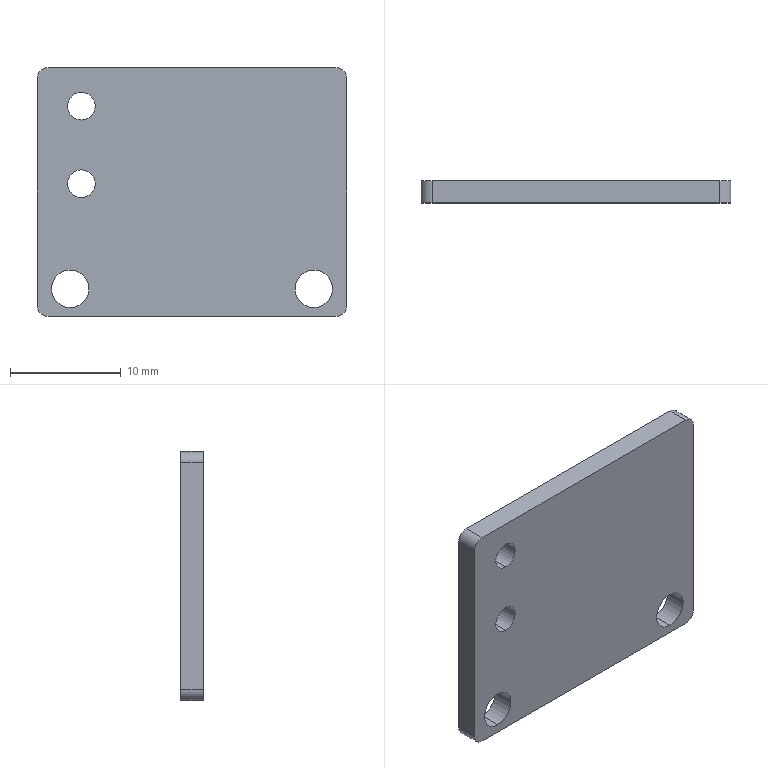Part | NX | features BREP 1 | 1 solid | 18 faces | box 28 x 2 x 22.5 mm | volume 1202 mm3 | cylinder 12 | plane 6 | commonest cylinder face diameters 2 x4 2.5 x4 3.4 x4
STEP:
#1=CARTESIAN_POINT('',(-28.,2.,21.5));
#2=VERTEX_POINT('',#1);
#3=CARTESIAN_POINT('',(-27.,2.,22.5));
#4=VERTEX_POINT('',#3);
#5=CARTESIAN_POINT('',(-27.,2.,21.5));
#6=DIRECTION('',(0.,1.,0.));
#7=DIRECTION('',(0.,0.,1.));
#8=AXIS2_PLACEMENT_3D('',#5,#6,#7);
#9=CIRCLE('',#8,1.);
#10=EDGE_CURVE('',#2,#4,#9,.T.);
#11=ORIENTED_EDGE('',*,*,#10,.F.);
#12=CARTESIAN_POINT('',(-28.,0.,21.5));
#13=VERTEX_POINT('',#12);
#14=CARTESIAN_POINT('',(-28.,2.,21.5));
#15=DIRECTION('',(0.,1.,0.));
#16=VECTOR('',#15,1000.);
#17=LINE('',#14,#16);
#18=EDGE_CURVE('',#13,#2,#17,.T.);
#19=ORIENTED_EDGE('',*,*,#18,.F.);
#20=CARTESIAN_POINT('',(-27.,0.,22.5));
#21=VERTEX_POINT('',#20);
#22=CARTESIAN_POINT('',(-27.,0.,21.5));
#23=DIRECTION('',(0.,-1.,0.));
#24=DIRECTION('',(0.,0.,1.));
#25=AXIS2_PLACEMENT_3D('',#22,#23,#24);
#26=CIRCLE('',#25,1.);
#27=EDGE_CURVE('',#21,#13,#26,.T.);
#28=ORIENTED_EDGE('',*,*,#27,.F.);
#29=CARTESIAN_POINT('',(-27.,0.,22.5));
#30=DIRECTION('',(0.,-1.,0.));
#31=VECTOR('',#30,1000.);
#32=LINE('',#29,#31);
#33=EDGE_CURVE('',#4,#21,#32,.T.);
#34=ORIENTED_EDGE('',*,*,#33,.F.);
#35=EDGE_LOOP('',(#11,#19,#28,#34));
#36=FACE_BOUND('',#35,.T.);
#37=CARTESIAN_POINT('',(-27.,2.,21.5));
#38=DIRECTION('',(0.,1.,0.));
#39=DIRECTION('',(0.,0.,1.));
#40=AXIS2_PLACEMENT_3D('',#37,#38,#39);
#41=CYLINDRICAL_SURFACE('',#40,1.);
#42=ADVANCED_FACE('',(#36),#41,.T.);
#43=CARTESIAN_POINT('',(-27.,2.,0.));
#44=VERTEX_POINT('',#43);
#45=CARTESIAN_POINT('',(-28.,2.,1.));
#46=VERTEX_POINT('',#45);
#47=CARTESIAN_POINT('',(-27.,2.,1.));
#48=DIRECTION('',(0.,1.,0.));
#49=DIRECTION('',(0.,0.,1.));
#50=AXIS2_PLACEMENT_3D('',#47,#48,#49);
#51=CIRCLE('',#50,1.);
#52=EDGE_CURVE('',#44,#46,#51,.T.);
#53=ORIENTED_EDGE('',*,*,#52,.F.);
#54=CARTESIAN_POINT('',(-27.,0.,0.));
#55=VERTEX_POINT('',#54);
#56=CARTESIAN_POINT('',(-27.,2.,0.));
#57=DIRECTION('',(0.,1.,0.));
#58=VECTOR('',#57,1000.);
#59=LINE('',#56,#58);
#60=EDGE_CURVE('',#55,#44,#59,.T.);
#61=ORIENTED_EDGE('',*,*,#60,.F.);
#62=CARTESIAN_POINT('',(-28.,0.,1.));
#63=VERTEX_POINT('',#62);
#64=CARTESIAN_POINT('',(-27.,0.,1.));
#65=DIRECTION('',(0.,-1.,0.));
#66=DIRECTION('',(0.,0.,1.));
#67=AXIS2_PLACEMENT_3D('',#64,#65,#66);
#68=CIRCLE('',#67,1.);
#69=EDGE_CURVE('',#63,#55,#68,.T.);
#70=ORIENTED_EDGE('',*,*,#69,.F.);
#71=CARTESIAN_POINT('',(-28.,2.,1.));
#72=DIRECTION('',(0.,-1.,0.));
#73=VECTOR('',#72,1000.);
#74=LINE('',#71,#73);
#75=EDGE_CURVE('',#46,#63,#74,.T.);
#76=ORIENTED_EDGE('',*,*,#75,.F.);
#77=EDGE_LOOP('',(#53,#61,#70,#76));
#78=FACE_BOUND('',#77,.T.);
#79=CARTESIAN_POINT('',(-27.,2.,1.));
#80=DIRECTION('',(0.,-1.,0.));
#81=DIRECTION('',(0.,0.,-1.));
#82=AXIS2_PLACEMENT_3D('',#79,#80,#81);
#83=CYLINDRICAL_SURFACE('',#82,1.);
#84=ADVANCED_FACE('',(#78),#83,.T.);
#85=CARTESIAN_POINT('',(-1.,2.,22.5));
#86=VERTEX_POINT('',#85);
#87=CARTESIAN_POINT('',(0.,2.,21.5));
#88=VERTEX_POINT('',#87);
#89=CARTESIAN_POINT('',(-1.,2.,21.5));
#90=DIRECTION('',(0.,1.,0.));
#91=DIRECTION('',(0.,0.,1.));
#92=AXIS2_PLACEMENT_3D('',#89,#90,#91);
#93=CIRCLE('',#92,1.);
#94=EDGE_CURVE('',#86,#88,#93,.T.);
#95=ORIENTED_EDGE('',*,*,#94,.F.);
#96=CARTESIAN_POINT('',(-1.,0.,22.5));
#97=VERTEX_POINT('',#96);
#98=CARTESIAN_POINT('',(-1.,2.,22.5));
#99=DIRECTION('',(0.,1.,0.));
#100=VECTOR('',#99,1000.);
#101=LINE('',#98,#100);
#102=EDGE_CURVE('',#97,#86,#101,.T.);
#103=ORIENTED_EDGE('',*,*,#102,.F.);
#104=CARTESIAN_POINT('',(0.,0.,21.5));
#105=VERTEX_POINT('',#104);
#106=CARTESIAN_POINT('',(-1.,0.,21.5));
#107=DIRECTION('',(0.,-1.,0.));
#108=DIRECTION('',(0.,0.,1.));
#109=AXIS2_PLACEMENT_3D('',#106,#107,#108);
#110=CIRCLE('',#109,1.);
#111=EDGE_CURVE('',#105,#97,#110,.T.);
#112=ORIENTED_EDGE('',*,*,#111,.F.);
#113=CARTESIAN_POINT('',(0.,2.,21.5));
#114=DIRECTION('',(0.,-1.,0.));
#115=VECTOR('',#114,1000.);
#116=LINE('',#113,#115);
#117=EDGE_CURVE('',#88,#105,#116,.T.);
#118=ORIENTED_EDGE('',*,*,#117,.F.);
#119=EDGE_LOOP('',(#95,#103,#112,#118));
#120=FACE_BOUND('',#119,.T.);
#121=CARTESIAN_POINT('',(-1.,2.,21.5));
#122=DIRECTION('',(0.,-1.,0.));
#123=DIRECTION('',(0.,0.,-1.));
#124=AXIS2_PLACEMENT_3D('',#121,#122,#123);
#125=CYLINDRICAL_SURFACE('',#124,1.);
#126=ADVANCED_FACE('',(#120),#125,.T.);
#127=CARTESIAN_POINT('',(0.,2.,1.));
#128=VERTEX_POINT('',#127);
#129=CARTESIAN_POINT('',(-1.,2.,0.));
#130=VERTEX_POINT('',#129);
#131=CARTESIAN_POINT('',(-1.,2.,1.));
#132=DIRECTION('',(0.,1.,0.));
#133=DIRECTION('',(0.,0.,1.));
#134=AXIS2_PLACEMENT_3D('',#131,#132,#133);
#135=CIRCLE('',#134,1.);
#136=EDGE_CURVE('',#128,#130,#135,.T.);
#137=ORIENTED_EDGE('',*,*,#136,.F.);
#138=CARTESIAN_POINT('',(0.,0.,1.));
#139=VERTEX_POINT('',#138);
#140=CARTESIAN_POINT('',(0.,2.,1.));
#141=DIRECTION('',(0.,1.,0.));
#142=VECTOR('',#141,1000.);
#143=LINE('',#140,#142);
#144=EDGE_CURVE('',#139,#128,#143,.T.);
#145=ORIENTED_EDGE('',*,*,#144,.F.);
#146=CARTESIAN_POINT('',(-1.,0.,0.));
#147=VERTEX_POINT('',#146);
#148=CARTESIAN_POINT('',(-1.,0.,1.));
#149=DIRECTION('',(0.,-1.,0.));
#150=DIRECTION('',(0.,0.,1.));
#151=AXIS2_PLACEMENT_3D('',#148,#149,#150);
#152=CIRCLE('',#151,1.);
#153=EDGE_CURVE('',#147,#139,#152,.T.);
#154=ORIENTED_EDGE('',*,*,#153,.F.);
#155=CARTESIAN_POINT('',(-1.,0.,0.));
#156=DIRECTION('',(0.,-1.,0.));
#157=VECTOR('',#156,1000.);
#158=LINE('',#155,#157);
#159=EDGE_CURVE('',#130,#147,#158,.T.);
#160=ORIENTED_EDGE('',*,*,#159,.F.);
#161=EDGE_LOOP('',(#137,#145,#154,#160));
#162=FACE_BOUND('',#161,.T.);
#163=CARTESIAN_POINT('',(-1.,2.,1.));
#164=DIRECTION('',(0.,1.,0.));
#165=DIRECTION('',(0.,0.,1.));
#166=AXIS2_PLACEMENT_3D('',#163,#164,#165);
#167=CYLINDRICAL_SURFACE('',#166,1.);
#168=ADVANCED_FACE('',(#162),#167,.T.);
#169=CARTESIAN_POINT('',(-24.,2.,10.75));
#170=VERTEX_POINT('',#169);
#171=CARTESIAN_POINT('',(-24.,0.,10.75));
#172=VERTEX_POINT('',#171);
#173=CARTESIAN_POINT('',(-24.,2.,10.75));
#174=DIRECTION('',(0.,1.,0.));
#175=VECTOR('',#174,1000.);
#176=LINE('',#173,#175);
#177=EDGE_CURVE('',#170,#172,#176,.F.);
#178=ORIENTED_EDGE('',*,*,#177,.T.);
#179=CARTESIAN_POINT('',(-24.,0.,13.25));
#180=VERTEX_POINT('',#179);
#181=CARTESIAN_POINT('',(-24.,0.,12.));
#182=DIRECTION('',(0.,1.,0.));
#183=DIRECTION('',(0.,0.,1.));
#184=AXIS2_PLACEMENT_3D('',#181,#182,#183);
#185=CIRCLE('',#184,1.25);
#186=EDGE_CURVE('',#180,#172,#185,.T.);
#187=ORIENTED_EDGE('',*,*,#186,.F.);
#188=CARTESIAN_POINT('',(-24.,2.,13.25));
#189=VERTEX_POINT('',#188);
#190=CARTESIAN_POINT('',(-24.,2.,13.25));
#191=DIRECTION('',(0.,1.,0.));
#192=VECTOR('',#191,1000.);
#193=LINE('',#190,#192);
#194=EDGE_CURVE('',#189,#180,#193,.F.);
#195=ORIENTED_EDGE('',*,*,#194,.F.);
#196=CARTESIAN_POINT('',(-24.,2.,12.));
#197=DIRECTION('',(0.,1.,0.));
#198=DIRECTION('',(0.,0.,1.));
#199=AXIS2_PLACEMENT_3D('',#196,#197,#198);
#200=CIRCLE('',#199,1.25);
#201=EDGE_CURVE('',#189,#170,#200,.T.);
#202=ORIENTED_EDGE('',*,*,#201,.T.);
#203=EDGE_LOOP('',(#178,#187,#195,#202));
#204=FACE_BOUND('',#203,.T.);
#205=CARTESIAN_POINT('',(-24.,2.,12.));
#206=DIRECTION('',(0.,1.,0.));
#207=DIRECTION('',(0.,0.,1.));
#208=AXIS2_PLACEMENT_3D('',#205,#206,#207);
#209=CYLINDRICAL_SURFACE('',#208,1.25);
#210=ADVANCED_FACE('',(#204),#209,.F.);
#211=CARTESIAN_POINT('',(-24.,2.,17.75));
#212=VERTEX_POINT('',#211);
#213=CARTESIAN_POINT('',(-24.,0.,17.75));
#214=VERTEX_POINT('',#213);
#215=CARTESIAN_POINT('',(-24.,2.,17.75));
#216=DIRECTION('',(0.,1.,0.));
#217=VECTOR('',#216,1000.);
#218=LINE('',#215,#217);
#219=EDGE_CURVE('',#212,#214,#218,.F.);
#220=ORIENTED_EDGE('',*,*,#219,.T.);
#221=CARTESIAN_POINT('',(-24.,0.,20.25));
#222=VERTEX_POINT('',#221);
#223=CARTESIAN_POINT('',(-24.,0.,19.));
#224=DIRECTION('',(0.,1.,0.));
#225=DIRECTION('',(0.,0.,1.));
#226=AXIS2_PLACEMENT_3D('',#223,#224,#225);
#227=CIRCLE('',#226,1.25);
#228=EDGE_CURVE('',#222,#214,#227,.T.);
#229=ORIENTED_EDGE('',*,*,#228,.F.);
#230=CARTESIAN_POINT('',(-24.,2.,20.25));
#231=VERTEX_POINT('',#230);
#232=CARTESIAN_POINT('',(-24.,2.,20.25));
#233=DIRECTION('',(0.,1.,0.));
#234=VECTOR('',#233,1000.);
#235=LINE('',#232,#234);
#236=EDGE_CURVE('',#231,#222,#235,.F.);
#237=ORIENTED_EDGE('',*,*,#236,.F.);
#238=CARTESIAN_POINT('',(-24.,2.,19.));
#239=DIRECTION('',(0.,1.,0.));
#240=DIRECTION('',(0.,0.,1.));
#241=AXIS2_PLACEMENT_3D('',#238,#239,#240);
#242=CIRCLE('',#241,1.25);
#243=EDGE_CURVE('',#231,#212,#242,.T.);
#244=ORIENTED_EDGE('',*,*,#243,.T.);
#245=EDGE_LOOP('',(#220,#229,#237,#244));
#246=FACE_BOUND('',#245,.T.);
#247=CARTESIAN_POINT('',(-24.,2.,19.));
#248=DIRECTION('',(0.,1.,0.));
#249=DIRECTION('',(0.,0.,1.));
#250=AXIS2_PLACEMENT_3D('',#247,#248,#249);
#251=CYLINDRICAL_SURFACE('',#250,1.25);
#252=ADVANCED_FACE('',(#246),#251,.F.);
#253=CARTESIAN_POINT('',(-25.,2.,0.8));
#254=VERTEX_POINT('',#253);
#255=CARTESIAN_POINT('',(-25.,0.,0.8));
#256=VERTEX_POINT('',#255);
#257=CARTESIAN_POINT('',(-25.,2.,0.8));
#258=DIRECTION('',(0.,1.,0.));
#259=VECTOR('',#258,1000.);
#260=LINE('',#257,#259);
#261=EDGE_CURVE('',#254,#256,#260,.F.);
#262=ORIENTED_EDGE('',*,*,#261,.T.);
#263=CARTESIAN_POINT('',(-25.,0.,4.2));
#264=VERTEX_POINT('',#263);
#265=CARTESIAN_POINT('',(-25.,0.,2.5));
#266=DIRECTION('',(0.,1.,0.));
#267=DIRECTION('',(0.,0.,1.));
#268=AXIS2_PLACEMENT_3D('',#265,#266,#267);
#269=CIRCLE('',#268,1.7);
#270=EDGE_CURVE('',#264,#256,#269,.T.);
#271=ORIENTED_EDGE('',*,*,#270,.F.);
#272=CARTESIAN_POINT('',(-25.,2.,4.2));
#273=VERTEX_POINT('',#272);
#274=CARTESIAN_POINT('',(-25.,2.,4.2));
#275=DIRECTION('',(0.,1.,0.));
#276=VECTOR('',#275,1000.);
#277=LINE('',#274,#276);
#278=EDGE_CURVE('',#273,#264,#277,.F.);
#279=ORIENTED_EDGE('',*,*,#278,.F.);
#280=CARTESIAN_POINT('',(-25.,2.,2.5));
#281=DIRECTION('',(0.,1.,0.));
#282=DIRECTION('',(0.,0.,1.));
#283=AXIS2_PLACEMENT_3D('',#280,#281,#282);
#284=CIRCLE('',#283,1.7);
#285=EDGE_CURVE('',#273,#254,#284,.T.);
#286=ORIENTED_EDGE('',*,*,#285,.T.);
#287=EDGE_LOOP('',(#262,#271,#279,#286));
#288=FACE_BOUND('',#287,.T.);
#289=CARTESIAN_POINT('',(-25.,2.,2.5));
#290=DIRECTION('',(0.,1.,0.));
#291=DIRECTION('',(0.,0.,1.));
#292=AXIS2_PLACEMENT_3D('',#289,#290,#291);
#293=CYLINDRICAL_SURFACE('',#292,1.7);
#294=ADVANCED_FACE('',(#288),#293,.F.);
#295=CARTESIAN_POINT('',(-3.,2.,0.8));
#296=VERTEX_POINT('',#295);
#297=CARTESIAN_POINT('',(-3.,0.,0.8));
#298=VERTEX_POINT('',#297);
#299=CARTESIAN_POINT('',(-3.,2.,0.8));
#300=DIRECTION('',(0.,1.,0.));
#301=VECTOR('',#300,1000.);
#302=LINE('',#299,#301);
#303=EDGE_CURVE('',#296,#298,#302,.F.);
#304=ORIENTED_EDGE('',*,*,#303,.T.);
#305=CARTESIAN_POINT('',(-3.,0.,4.2));
#306=VERTEX_POINT('',#305);
#307=CARTESIAN_POINT('',(-3.,0.,2.5));
#308=DIRECTION('',(0.,1.,0.));
#309=DIRECTION('',(0.,0.,1.));
#310=AXIS2_PLACEMENT_3D('',#307,#308,#309);
#311=CIRCLE('',#310,1.7);
#312=EDGE_CURVE('',#306,#298,#311,.T.);
#313=ORIENTED_EDGE('',*,*,#312,.F.);
#314=CARTESIAN_POINT('',(-3.,2.,4.2));
#315=VERTEX_POINT('',#314);
#316=CARTESIAN_POINT('',(-3.,2.,4.2));
#317=DIRECTION('',(0.,1.,0.));
#318=VECTOR('',#317,1000.);
#319=LINE('',#316,#318);
#320=EDGE_CURVE('',#315,#306,#319,.F.);
#321=ORIENTED_EDGE('',*,*,#320,.F.);
#322=CARTESIAN_POINT('',(-3.,2.,2.5));
#323=DIRECTION('',(0.,1.,0.));
#324=DIRECTION('',(0.,0.,1.));
#325=AXIS2_PLACEMENT_3D('',#322,#323,#324);
#326=CIRCLE('',#325,1.7);
#327=EDGE_CURVE('',#315,#296,#326,.T.);
#328=ORIENTED_EDGE('',*,*,#327,.T.);
#329=EDGE_LOOP('',(#304,#313,#321,#328));
#330=FACE_BOUND('',#329,.T.);
#331=CARTESIAN_POINT('',(-3.,2.,2.5));
#332=DIRECTION('',(0.,1.,0.));
#333=DIRECTION('',(0.,0.,1.));
#334=AXIS2_PLACEMENT_3D('',#331,#332,#333);
#335=CYLINDRICAL_SURFACE('',#334,1.7);
#336=ADVANCED_FACE('',(#330),#335,.F.);
#337=CARTESIAN_POINT('',(0.,0.,0.));
#338=DIRECTION('',(-1.,0.,0.));
#339=VECTOR('',#338,1000.);
#340=LINE('',#337,#339);
#341=EDGE_CURVE('',#147,#55,#340,.T.);
#342=ORIENTED_EDGE('',*,*,#341,.F.);
#343=ORIENTED_EDGE('',*,*,#153,.T.);
#344=CARTESIAN_POINT('',(0.,0.,0.));
#345=DIRECTION('',(0.,0.,1.));
#346=VECTOR('',#345,1000.);
#347=LINE('',#344,#346);
#348=EDGE_CURVE('',#139,#105,#347,.T.);
#349=ORIENTED_EDGE('',*,*,#348,.T.);
#350=ORIENTED_EDGE('',*,*,#111,.T.);
#351=CARTESIAN_POINT('',(0.,0.,22.5));
#352=DIRECTION('',(-1.,0.,0.));
#353=VECTOR('',#352,1000.);
#354=LINE('',#351,#353);
#355=EDGE_CURVE('',#97,#21,#354,.T.);
#356=ORIENTED_EDGE('',*,*,#355,.T.);
#357=ORIENTED_EDGE('',*,*,#27,.T.);
#358=CARTESIAN_POINT('',(-28.,0.,0.));
#359=DIRECTION('',(0.,0.,1.));
#360=VECTOR('',#359,1000.);
#361=LINE('',#358,#360);
#362=EDGE_CURVE('',#63,#13,#361,.T.);
#363=ORIENTED_EDGE('',*,*,#362,.F.);
#364=ORIENTED_EDGE('',*,*,#69,.T.);
#365=EDGE_LOOP('',(#342,#343,#349,#350,#356,#357,#363,#364));
#366=FACE_BOUND('',#365,.T.);
#367=ORIENTED_EDGE('',*,*,#312,.T.);
#368=CARTESIAN_POINT('',(-3.,0.,2.5));
#369=DIRECTION('',(0.,1.,0.));
#370=DIRECTION('',(0.,0.,1.));
#371=AXIS2_PLACEMENT_3D('',#368,#369,#370);
#372=CIRCLE('',#371,1.7);
#373=EDGE_CURVE('',#298,#306,#372,.T.);
#374=ORIENTED_EDGE('',*,*,#373,.T.);
#375=EDGE_LOOP('',(#367,#374));
#376=FACE_BOUND('',#375,.T.);
#377=ORIENTED_EDGE('',*,*,#270,.T.);
#378=CARTESIAN_POINT('',(-25.,0.,2.5));
#379=DIRECTION('',(0.,1.,0.));
#380=DIRECTION('',(0.,0.,1.));
#381=AXIS2_PLACEMENT_3D('',#378,#379,#380);
#382=CIRCLE('',#381,1.7);
#383=EDGE_CURVE('',#256,#264,#382,.T.);
#384=ORIENTED_EDGE('',*,*,#383,.T.);
#385=EDGE_LOOP('',(#377,#384));
#386=FACE_BOUND('',#385,.T.);
#387=ORIENTED_EDGE('',*,*,#228,.T.);
#388=CARTESIAN_POINT('',(-24.,0.,19.));
#389=DIRECTION('',(0.,1.,0.));
#390=DIRECTION('',(0.,0.,1.));
#391=AXIS2_PLACEMENT_3D('',#388,#389,#390);
#392=CIRCLE('',#391,1.25);
#393=EDGE_CURVE('',#214,#222,#392,.T.);
#394=ORIENTED_EDGE('',*,*,#393,.T.);
#395=EDGE_LOOP('',(#387,#394));
#396=FACE_BOUND('',#395,.T.);
#397=ORIENTED_EDGE('',*,*,#186,.T.);
#398=CARTESIAN_POINT('',(-24.,0.,12.));
#399=DIRECTION('',(0.,1.,0.));
#400=DIRECTION('',(0.,0.,1.));
#401=AXIS2_PLACEMENT_3D('',#398,#399,#400);
#402=CIRCLE('',#401,1.25);
#403=EDGE_CURVE('',#172,#180,#402,.T.);
#404=ORIENTED_EDGE('',*,*,#403,.T.);
#405=EDGE_LOOP('',(#397,#404));
#406=FACE_BOUND('',#405,.T.);
#407=CARTESIAN_POINT('',(0.,0.,0.));
#408=DIRECTION('',(0.,1.,0.));
#409=DIRECTION('',(0.,0.,1.));
#410=AXIS2_PLACEMENT_3D('',#407,#408,#409);
#411=PLANE('',#410);
#412=ADVANCED_FACE('',(#366,#376,#386,#396,#406),#411,.F.);
#413=CARTESIAN_POINT('',(0.,2.,0.));
#414=DIRECTION('',(0.,0.,1.));
#415=VECTOR('',#414,1000.);
#416=LINE('',#413,#415);
#417=EDGE_CURVE('',#128,#88,#416,.T.);
#418=ORIENTED_EDGE('',*,*,#417,.F.);
#419=ORIENTED_EDGE('',*,*,#136,.T.);
#420=CARTESIAN_POINT('',(0.,2.,0.));
#421=DIRECTION('',(-1.,0.,0.));
#422=VECTOR('',#421,1000.);
#423=LINE('',#420,#422);
#424=EDGE_CURVE('',#130,#44,#423,.T.);
#425=ORIENTED_EDGE('',*,*,#424,.T.);
#426=ORIENTED_EDGE('',*,*,#52,.T.);
#427=CARTESIAN_POINT('',(-28.,2.,0.));
#428=DIRECTION('',(0.,0.,1.));
#429=VECTOR('',#428,1000.);
#430=LINE('',#427,#429);
#431=EDGE_CURVE('',#46,#2,#430,.T.);
#432=ORIENTED_EDGE('',*,*,#431,.T.);
#433=ORIENTED_EDGE('',*,*,#10,.T.);
#434=CARTESIAN_POINT('',(0.,2.,22.5));
#435=DIRECTION('',(-1.,0.,0.));
#436=VECTOR('',#435,1000.);
#437=LINE('',#434,#436);
#438=EDGE_CURVE('',#86,#4,#437,.T.);
#439=ORIENTED_EDGE('',*,*,#438,.F.);
#440=ORIENTED_EDGE('',*,*,#94,.T.);
#441=EDGE_LOOP('',(#418,#419,#425,#426,#432,#433,#439,#440));
#442=FACE_BOUND('',#441,.T.);
#443=ORIENTED_EDGE('',*,*,#327,.F.);
#444=CARTESIAN_POINT('',(-3.,2.,2.5));
#445=DIRECTION('',(0.,1.,0.));
#446=DIRECTION('',(0.,0.,1.));
#447=AXIS2_PLACEMENT_3D('',#444,#445,#446);
#448=CIRCLE('',#447,1.7);
#449=EDGE_CURVE('',#296,#315,#448,.T.);
#450=ORIENTED_EDGE('',*,*,#449,.F.);
#451=EDGE_LOOP('',(#443,#450));
#452=FACE_BOUND('',#451,.T.);
#453=ORIENTED_EDGE('',*,*,#285,.F.);
#454=CARTESIAN_POINT('',(-25.,2.,2.5));
#455=DIRECTION('',(0.,1.,0.));
#456=DIRECTION('',(0.,0.,1.));
#457=AXIS2_PLACEMENT_3D('',#454,#455,#456);
#458=CIRCLE('',#457,1.7);
#459=EDGE_CURVE('',#254,#273,#458,.T.);
#460=ORIENTED_EDGE('',*,*,#459,.F.);
#461=EDGE_LOOP('',(#453,#460));
#462=FACE_BOUND('',#461,.T.);
#463=ORIENTED_EDGE('',*,*,#243,.F.);
#464=CARTESIAN_POINT('',(-24.,2.,19.));
#465=DIRECTION('',(0.,1.,0.));
#466=DIRECTION('',(0.,0.,1.));
#467=AXIS2_PLACEMENT_3D('',#464,#465,#466);
#468=CIRCLE('',#467,1.25);
#469=EDGE_CURVE('',#212,#231,#468,.T.);
#470=ORIENTED_EDGE('',*,*,#469,.F.);
#471=EDGE_LOOP('',(#463,#470));
#472=FACE_BOUND('',#471,.T.);
#473=ORIENTED_EDGE('',*,*,#201,.F.);
#474=CARTESIAN_POINT('',(-24.,2.,12.));
#475=DIRECTION('',(0.,1.,0.));
#476=DIRECTION('',(0.,0.,1.));
#477=AXIS2_PLACEMENT_3D('',#474,#475,#476);
#478=CIRCLE('',#477,1.25);
#479=EDGE_CURVE('',#170,#189,#478,.T.);
#480=ORIENTED_EDGE('',*,*,#479,.F.);
#481=EDGE_LOOP('',(#473,#480));
#482=FACE_BOUND('',#481,.T.);
#483=CARTESIAN_POINT('',(0.,2.,0.));
#484=DIRECTION('',(0.,1.,0.));
#485=DIRECTION('',(0.,0.,1.));
#486=AXIS2_PLACEMENT_3D('',#483,#484,#485);
#487=PLANE('',#486);
#488=ADVANCED_FACE('',(#442,#452,#462,#472,#482),#487,.T.);
#489=ORIENTED_EDGE('',*,*,#348,.F.);
#490=ORIENTED_EDGE('',*,*,#144,.T.);
#491=ORIENTED_EDGE('',*,*,#417,.T.);
#492=ORIENTED_EDGE('',*,*,#117,.T.);
#493=EDGE_LOOP('',(#489,#490,#491,#492));
#494=FACE_BOUND('',#493,.T.);
#495=CARTESIAN_POINT('',(0.,2.,0.));
#496=DIRECTION('',(1.,0.,0.));
#497=DIRECTION('',(0.,0.,-1.));
#498=AXIS2_PLACEMENT_3D('',#495,#496,#497);
#499=PLANE('',#498);
#500=ADVANCED_FACE('',(#494),#499,.T.);
#501=ORIENTED_EDGE('',*,*,#355,.F.);
#502=ORIENTED_EDGE('',*,*,#102,.T.);
#503=ORIENTED_EDGE('',*,*,#438,.T.);
#504=ORIENTED_EDGE('',*,*,#33,.T.);
#505=EDGE_LOOP('',(#501,#502,#503,#504));
#506=FACE_BOUND('',#505,.T.);
#507=CARTESIAN_POINT('',(0.,2.,22.5));
#508=DIRECTION('',(0.,0.,1.));
#509=DIRECTION('',(1.,0.,0.));
#510=AXIS2_PLACEMENT_3D('',#507,#508,#509);
#511=PLANE('',#510);
#512=ADVANCED_FACE('',(#506),#511,.T.);
#513=ORIENTED_EDGE('',*,*,#431,.F.);
#514=ORIENTED_EDGE('',*,*,#75,.T.);
#515=ORIENTED_EDGE('',*,*,#362,.T.);
#516=ORIENTED_EDGE('',*,*,#18,.T.);
#517=EDGE_LOOP('',(#513,#514,#515,#516));
#518=FACE_BOUND('',#517,.T.);
#519=CARTESIAN_POINT('',(-28.,2.,0.));
#520=DIRECTION('',(1.,0.,0.));
#521=DIRECTION('',(0.,0.,-1.));
#522=AXIS2_PLACEMENT_3D('',#519,#520,#521);
#523=PLANE('',#522);
#524=ADVANCED_FACE('',(#518),#523,.F.);
#525=ORIENTED_EDGE('',*,*,#424,.F.);
#526=ORIENTED_EDGE('',*,*,#159,.T.);
#527=ORIENTED_EDGE('',*,*,#341,.T.);
#528=ORIENTED_EDGE('',*,*,#60,.T.);
#529=EDGE_LOOP('',(#525,#526,#527,#528));
#530=FACE_BOUND('',#529,.T.);
#531=CARTESIAN_POINT('',(0.,2.,0.));
#532=DIRECTION('',(0.,0.,1.));
#533=DIRECTION('',(1.,0.,0.));
#534=AXIS2_PLACEMENT_3D('',#531,#532,#533);
#535=PLANE('',#534);
#536=ADVANCED_FACE('',(#530),#535,.F.);
#537=ORIENTED_EDGE('',*,*,#373,.F.);
#538=ORIENTED_EDGE('',*,*,#303,.F.);
#539=ORIENTED_EDGE('',*,*,#449,.T.);
#540=ORIENTED_EDGE('',*,*,#320,.T.);
#541=EDGE_LOOP('',(#537,#538,#539,#540));
#542=FACE_BOUND('',#541,.T.);
#543=CARTESIAN_POINT('',(-3.,2.,2.5));
#544=DIRECTION('',(0.,1.,0.));
#545=DIRECTION('',(0.,0.,1.));
#546=AXIS2_PLACEMENT_3D('',#543,#544,#545);
#547=CYLINDRICAL_SURFACE('',#546,1.7);
#548=ADVANCED_FACE('',(#542),#547,.F.);
#549=ORIENTED_EDGE('',*,*,#383,.F.);
#550=ORIENTED_EDGE('',*,*,#261,.F.);
#551=ORIENTED_EDGE('',*,*,#459,.T.);
#552=ORIENTED_EDGE('',*,*,#278,.T.);
#553=EDGE_LOOP('',(#549,#550,#551,#552));
#554=FACE_BOUND('',#553,.T.);
#555=CARTESIAN_POINT('',(-25.,2.,2.5));
#556=DIRECTION('',(0.,1.,0.));
#557=DIRECTION('',(0.,0.,1.));
#558=AXIS2_PLACEMENT_3D('',#555,#556,#557);
#559=CYLINDRICAL_SURFACE('',#558,1.7);
#560=ADVANCED_FACE('',(#554),#559,.F.);
#561=ORIENTED_EDGE('',*,*,#393,.F.);
#562=ORIENTED_EDGE('',*,*,#219,.F.);
#563=ORIENTED_EDGE('',*,*,#469,.T.);
#564=ORIENTED_EDGE('',*,*,#236,.T.);
#565=EDGE_LOOP('',(#561,#562,#563,#564));
#566=FACE_BOUND('',#565,.T.);
#567=CARTESIAN_POINT('',(-24.,2.,19.));
#568=DIRECTION('',(0.,1.,0.));
#569=DIRECTION('',(0.,0.,1.));
#570=AXIS2_PLACEMENT_3D('',#567,#568,#569);
#571=CYLINDRICAL_SURFACE('',#570,1.25);
#572=ADVANCED_FACE('',(#566),#571,.F.);
#573=ORIENTED_EDGE('',*,*,#403,.F.);
#574=ORIENTED_EDGE('',*,*,#177,.F.);
#575=ORIENTED_EDGE('',*,*,#479,.T.);
#576=ORIENTED_EDGE('',*,*,#194,.T.);
#577=EDGE_LOOP('',(#573,#574,#575,#576));
#578=FACE_BOUND('',#577,.T.);
#579=CARTESIAN_POINT('',(-24.,2.,12.));
#580=DIRECTION('',(0.,1.,0.));
#581=DIRECTION('',(0.,0.,1.));
#582=AXIS2_PLACEMENT_3D('',#579,#580,#581);
#583=CYLINDRICAL_SURFACE('',#582,1.25);
#584=ADVANCED_FACE('',(#578),#583,.F.);
#585=CLOSED_SHELL('',(#42,#84,#126,#168,#210,#252,#294,#336,#412,#488,#500,#512,#524,#536,#548,#560,#572,#584));
#586=MANIFOLD_SOLID_BREP('',#585);
#587=(LENGTH_UNIT()NAMED_UNIT(*)SI_UNIT(.MILLI.,.METRE.));
#588=UNCERTAINTY_MEASURE_WITH_UNIT(LENGTH_MEASURE(0.00001),#587,'','');
#589=(NAMED_UNIT(*)PLANE_ANGLE_UNIT()SI_UNIT($,.RADIAN.));
#590=(NAMED_UNIT(*)SI_UNIT($,.STERADIAN.)SOLID_ANGLE_UNIT());
#591=(GEOMETRIC_REPRESENTATION_CONTEXT(3)GLOBAL_UNCERTAINTY_ASSIGNED_CONTEXT((#588))GLOBAL_UNIT_ASSIGNED_CONTEXT((#587,#589,#590))REPRESENTATION_CONTEXT('',''));
#592=ADVANCED_BREP_SHAPE_REPRESENTATION('',(#586),#591);